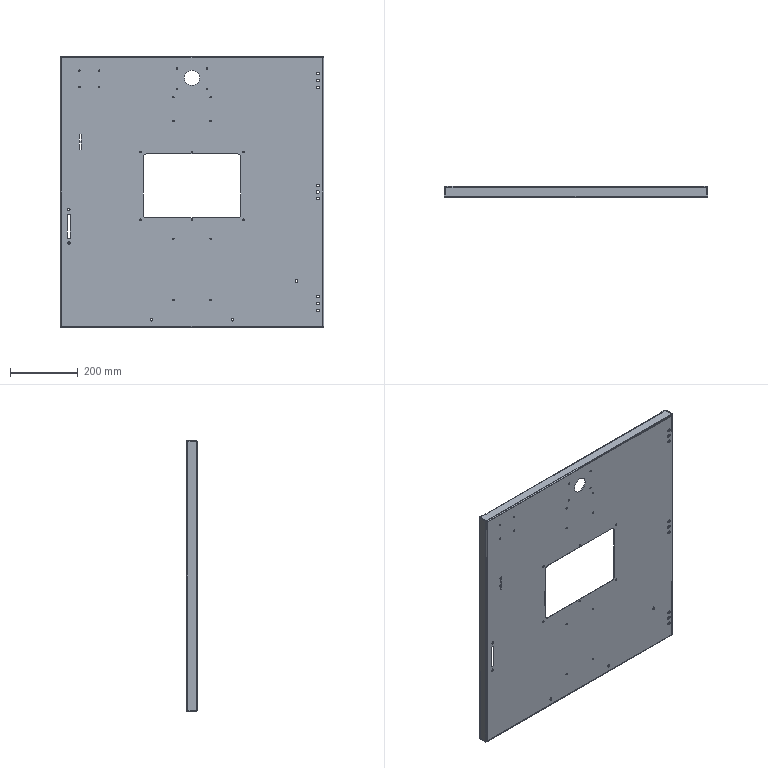Part | STEP file | 1 solid | 265 faces | box 775 x 32 x 796 mm | volume 1362848 mm3 | plane 161 | cylinder 104 | commonest cylinder face diameters 7 x34 4.2 x32 3 x12 5.3 x12 6.4 x6 20.5 x4